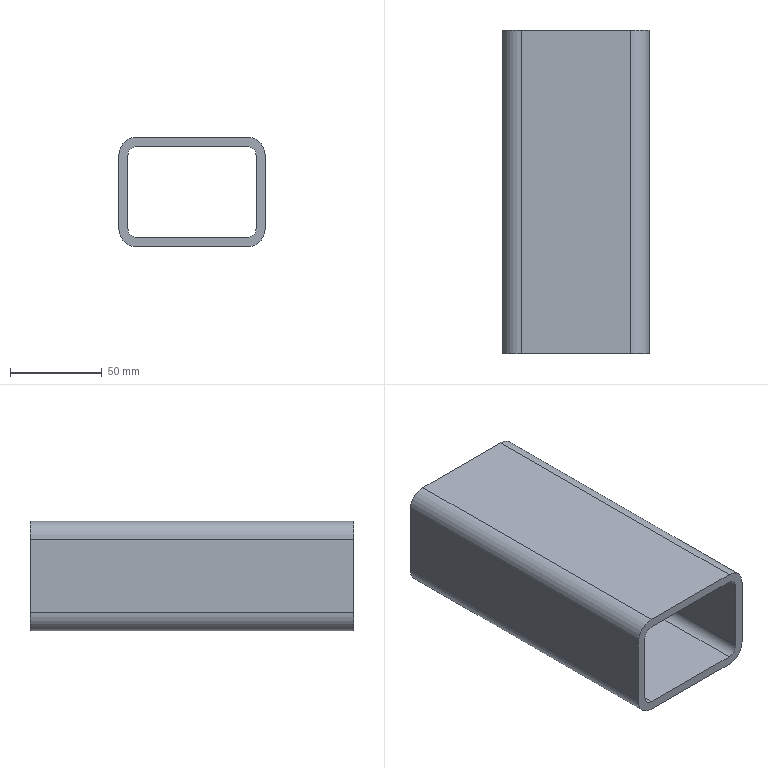Part | STEP file | front support crossmember--000.001--20240925 | 1 solid | 18 faces | box 80 x 176.5 x 60 mm | volume 218087 mm3 | plane 10 | cylinder 8 | commonest cylinder face diameters 10 x4 20 x4
STEP:
#1=CARTESIAN_POINT('',(0.,0.,0.));
#2=DIRECTION('',(0.,0.,1.));
#3=DIRECTION('',(1.,0.,0.));
#4=AXIS2_PLACEMENT_3D('',#1,#2,#3);
#5=CARTESIAN_POINT('',(10.,-176.5,40.));
#6=VERTEX_POINT('',#5);
#7=CARTESIAN_POINT('',(10.,-176.5,0.));
#8=VERTEX_POINT('',#7);
#9=CARTESIAN_POINT('',(10.,-176.5,20.));
#10=DIRECTION('',(0.,0.,-1.));
#11=VECTOR('',#10,1.);
#12=LINE('',#9,#11);
#13=CARTESIAN_POINT('',(10.,-76.5,20.));
#14=DIRECTION('',(1.,0.,0.));
#15=DIRECTION('',(0.,1.,0.));
#16=AXIS2_PLACEMENT_3D('',#13,#14,#15);
#17=PLANE('',#16);
#18=CARTESIAN_POINT('',(-100.,0.));
#19=DIRECTION('',(0.,-1.));
#20=VECTOR('',#19,1.);
#21=LINE('',#18,#20);
#22=(GEOMETRIC_REPRESENTATION_CONTEXT(2)PARAMETRIC_REPRESENTATION_CONTEXT()REPRESENTATION_CONTEXT('',''));
#23=DEFINITIONAL_REPRESENTATION('',(#21),#22);
#24=PCURVE('',#17,#23);
#25=CARTESIAN_POINT('',(-30.,-176.5,20.));
#26=DIRECTION('',(0.,-1.,0.));
#27=DIRECTION('',(1.,0.,0.));
#28=AXIS2_PLACEMENT_3D('',#25,#26,#27);
#29=PLANE('',#28);
#30=CARTESIAN_POINT('',(40.,0.));
#31=DIRECTION('',(0.,-1.));
#32=VECTOR('',#31,1.);
#33=LINE('',#30,#32);
#34=(GEOMETRIC_REPRESENTATION_CONTEXT(2)PARAMETRIC_REPRESENTATION_CONTEXT()REPRESENTATION_CONTEXT('',''));
#35=DEFINITIONAL_REPRESENTATION('',(#33),#34);
#36=PCURVE('',#29,#35);
#37=SURFACE_CURVE('',#12,(#24,#36),.PCURVE_S1.);
#38=EDGE_CURVE('',#6,#8,#37,.T.);
#39=ORIENTED_EDGE('',*,*,#38,.T.);
#40=CARTESIAN_POINT('',(10.,0.,0.));
#41=VERTEX_POINT('',#40);
#42=CARTESIAN_POINT('',(10.,-76.5,0.));
#43=DIRECTION('',(0.,1.,0.));
#44=VECTOR('',#43,1.);
#45=LINE('',#42,#44);
#46=CARTESIAN_POINT('',(0.,-20.));
#47=DIRECTION('',(1.,0.));
#48=VECTOR('',#47,1.);
#49=LINE('',#46,#48);
#50=(GEOMETRIC_REPRESENTATION_CONTEXT(2)PARAMETRIC_REPRESENTATION_CONTEXT()REPRESENTATION_CONTEXT('',''));
#51=DEFINITIONAL_REPRESENTATION('',(#49),#50);
#52=PCURVE('',#17,#51);
#53=CARTESIAN_POINT('',(0.,-76.5,0.));
#54=DIRECTION('',(0.,-1.,0.));
#55=DIRECTION('',(-0.06976,0.,-0.9976));
#56=AXIS2_PLACEMENT_3D('',#53,#54,#55);
#57=CYLINDRICAL_SURFACE('',#56,10.);
#58=CARTESIAN_POINT('',(1.641,0.));
#59=DIRECTION('',(0.,-1.));
#60=VECTOR('',#59,1.);
#61=LINE('',#58,#60);
#62=(GEOMETRIC_REPRESENTATION_CONTEXT(2)PARAMETRIC_REPRESENTATION_CONTEXT()REPRESENTATION_CONTEXT('',''));
#63=DEFINITIONAL_REPRESENTATION('',(#61),#62);
#64=PCURVE('',#57,#63);
#65=SURFACE_CURVE('',#45,(#52,#64),.PCURVE_S1.);
#66=EDGE_CURVE('',#8,#41,#65,.T.);
#67=ORIENTED_EDGE('',*,*,#66,.T.);
#68=CARTESIAN_POINT('',(10.,0.,40.));
#69=VERTEX_POINT('',#68);
#70=CARTESIAN_POINT('',(10.,0.,-87.645));
#71=DIRECTION('',(0.,0.,-1.));
#72=VECTOR('',#71,1.);
#73=LINE('',#70,#72);
#74=CARTESIAN_POINT('',(76.5,-107.645));
#75=DIRECTION('',(0.,-1.));
#76=VECTOR('',#75,1.);
#77=LINE('',#74,#76);
#78=(GEOMETRIC_REPRESENTATION_CONTEXT(2)PARAMETRIC_REPRESENTATION_CONTEXT()REPRESENTATION_CONTEXT('',''));
#79=DEFINITIONAL_REPRESENTATION('',(#77),#78);
#80=PCURVE('',#17,#79);
#81=CARTESIAN_POINT('',(131.5,0.,-87.645));
#82=DIRECTION('',(0.,1.,0.));
#83=DIRECTION('',(0.,0.,1.));
#84=AXIS2_PLACEMENT_3D('',#81,#82,#83);
#85=PLANE('',#84);
#86=CARTESIAN_POINT('',(0.,-121.5));
#87=DIRECTION('',(-1.,0.));
#88=VECTOR('',#87,1.);
#89=LINE('',#86,#88);
#90=(GEOMETRIC_REPRESENTATION_CONTEXT(2)PARAMETRIC_REPRESENTATION_CONTEXT()REPRESENTATION_CONTEXT('',''));
#91=DEFINITIONAL_REPRESENTATION('',(#89),#90);
#92=PCURVE('',#85,#91);
#93=SURFACE_CURVE('',#73,(#80,#92),.PCURVE_S1.);
#94=EDGE_CURVE('',#69,#41,#93,.T.);
#95=ORIENTED_EDGE('',*,*,#94,.F.);
#96=CARTESIAN_POINT('',(10.,-176.5,40.));
#97=DIRECTION('',(0.,-1.,0.));
#98=VECTOR('',#97,1.);
#99=LINE('',#96,#98);
#100=CARTESIAN_POINT('',(-100.,20.));
#101=DIRECTION('',(-1.,0.));
#102=VECTOR('',#101,1.);
#103=LINE('',#100,#102);
#104=(GEOMETRIC_REPRESENTATION_CONTEXT(2)PARAMETRIC_REPRESENTATION_CONTEXT()REPRESENTATION_CONTEXT('',''));
#105=DEFINITIONAL_REPRESENTATION('',(#103),#104);
#106=PCURVE('',#17,#105);
#107=CARTESIAN_POINT('',(0.,-76.5,40.));
#108=DIRECTION('',(0.,1.,0.));
#109=DIRECTION('',(0.06976,0.,0.9976));
#110=AXIS2_PLACEMENT_3D('',#107,#108,#109);
#111=CYLINDRICAL_SURFACE('',#110,10.);
#112=CARTESIAN_POINT('',(1.501,-100.));
#113=DIRECTION('',(0.,-1.));
#114=VECTOR('',#113,1.);
#115=LINE('',#112,#114);
#116=(GEOMETRIC_REPRESENTATION_CONTEXT(2)PARAMETRIC_REPRESENTATION_CONTEXT()REPRESENTATION_CONTEXT('',''));
#117=DEFINITIONAL_REPRESENTATION('',(#115),#116);
#118=PCURVE('',#111,#117);
#119=SURFACE_CURVE('',#99,(#106,#118),.PCURVE_S1.);
#120=EDGE_CURVE('',#69,#6,#119,.T.);
#121=ORIENTED_EDGE('',*,*,#120,.T.);
#122=EDGE_LOOP('',(#39,#67,#95,#121));
#123=FACE_BOUND('',#122,.T.);
#124=ADVANCED_FACE('',(#123),#17,.T.);
#125=CARTESIAN_POINT('',(-60.,-176.5,-5.));
#126=VERTEX_POINT('',#125);
#127=CARTESIAN_POINT('',(0.,-176.5,-5.));
#128=VERTEX_POINT('',#127);
#129=CARTESIAN_POINT('',(-30.,-176.5,-5.));
#130=DIRECTION('',(1.,0.,0.));
#131=VECTOR('',#130,1.);
#132=LINE('',#129,#131);
#133=CARTESIAN_POINT('',(0.,-25.));
#134=DIRECTION('',(1.,0.));
#135=VECTOR('',#134,1.);
#136=LINE('',#133,#135);
#137=(GEOMETRIC_REPRESENTATION_CONTEXT(2)PARAMETRIC_REPRESENTATION_CONTEXT()REPRESENTATION_CONTEXT('',''));
#138=DEFINITIONAL_REPRESENTATION('',(#136),#137);
#139=PCURVE('',#29,#138);
#140=CARTESIAN_POINT('',(-70.,-76.5,-5.));
#141=DIRECTION('',(0.,0.,-1.));
#142=DIRECTION('',(1.,0.,0.));
#143=AXIS2_PLACEMENT_3D('',#140,#141,#142);
#144=PLANE('',#143);
#145=CARTESIAN_POINT('',(40.,100.));
#146=DIRECTION('',(1.,0.));
#147=VECTOR('',#146,1.);
#148=LINE('',#145,#147);
#149=(GEOMETRIC_REPRESENTATION_CONTEXT(2)PARAMETRIC_REPRESENTATION_CONTEXT()REPRESENTATION_CONTEXT('',''));
#150=DEFINITIONAL_REPRESENTATION('',(#148),#149);
#151=PCURVE('',#144,#150);
#152=SURFACE_CURVE('',#132,(#139,#151),.PCURVE_S1.);
#153=EDGE_CURVE('',#126,#128,#152,.T.);
#154=ORIENTED_EDGE('',*,*,#153,.F.);
#155=CARTESIAN_POINT('',(-65.,-176.5,0.));
#156=VERTEX_POINT('',#155);
#157=CARTESIAN_POINT('',(-60.,-176.5,0.));
#158=DIRECTION('',(0.,-1.,0.));
#159=DIRECTION('',(0.06976,0.,0.9976));
#160=AXIS2_PLACEMENT_3D('',#157,#158,#159);
#161=CIRCLE('',#160,5.);
#162=CARTESIAN_POINT('',(-30.,-20.));
#163=DIRECTION('',(0.06976,0.9976));
#164=AXIS2_PLACEMENT_2D('',#162,#163);
#165=CIRCLE('',#164,5.);
#166=(GEOMETRIC_REPRESENTATION_CONTEXT(2)PARAMETRIC_REPRESENTATION_CONTEXT()REPRESENTATION_CONTEXT('',''));
#167=DEFINITIONAL_REPRESENTATION('',(#165),#166);
#168=PCURVE('',#29,#167);
#169=CARTESIAN_POINT('',(-60.,-76.5,0.));
#170=DIRECTION('',(0.,1.,0.));
#171=DIRECTION('',(0.06976,0.,0.9976));
#172=AXIS2_PLACEMENT_3D('',#169,#170,#171);
#173=CYLINDRICAL_SURFACE('',#172,5.);
#174=CARTESIAN_POINT('',(6.283,-100.));
#175=DIRECTION('',(-1.,0.));
#176=VECTOR('',#175,1.);
#177=LINE('',#174,#176);
#178=(GEOMETRIC_REPRESENTATION_CONTEXT(2)PARAMETRIC_REPRESENTATION_CONTEXT()REPRESENTATION_CONTEXT('',''));
#179=DEFINITIONAL_REPRESENTATION('',(#177),#178);
#180=PCURVE('',#173,#179);
#181=SURFACE_CURVE('',#161,(#168,#180),.PCURVE_S1.);
#182=EDGE_CURVE('',#156,#126,#181,.T.);
#183=ORIENTED_EDGE('',*,*,#182,.F.);
#184=CARTESIAN_POINT('',(-65.,-176.5,40.));
#185=VERTEX_POINT('',#184);
#186=CARTESIAN_POINT('',(-65.,-176.5,20.));
#187=DIRECTION('',(0.,0.,-1.));
#188=VECTOR('',#187,1.);
#189=LINE('',#186,#188);
#190=CARTESIAN_POINT('',(-35.,0.));
#191=DIRECTION('',(0.,-1.));
#192=VECTOR('',#191,1.);
#193=LINE('',#190,#192);
#194=(GEOMETRIC_REPRESENTATION_CONTEXT(2)PARAMETRIC_REPRESENTATION_CONTEXT()REPRESENTATION_CONTEXT('',''));
#195=DEFINITIONAL_REPRESENTATION('',(#193),#194);
#196=PCURVE('',#29,#195);
#197=CARTESIAN_POINT('',(-65.,-76.5,20.));
#198=DIRECTION('',(1.,0.,0.));
#199=DIRECTION('',(0.,1.,0.));
#200=AXIS2_PLACEMENT_3D('',#197,#198,#199);
#201=PLANE('',#200);
#202=CARTESIAN_POINT('',(-100.,0.));
#203=DIRECTION('',(0.,-1.));
#204=VECTOR('',#203,1.);
#205=LINE('',#202,#204);
#206=(GEOMETRIC_REPRESENTATION_CONTEXT(2)PARAMETRIC_REPRESENTATION_CONTEXT()REPRESENTATION_CONTEXT('',''));
#207=DEFINITIONAL_REPRESENTATION('',(#205),#206);
#208=PCURVE('',#201,#207);
#209=SURFACE_CURVE('',#189,(#196,#208),.PCURVE_S1.);
#210=EDGE_CURVE('',#185,#156,#209,.T.);
#211=ORIENTED_EDGE('',*,*,#210,.F.);
#212=CARTESIAN_POINT('',(-60.,-176.5,45.));
#213=VERTEX_POINT('',#212);
#214=CARTESIAN_POINT('',(-60.,-176.5,40.));
#215=DIRECTION('',(0.,-1.,0.));
#216=DIRECTION('',(0.06976,0.,0.9976));
#217=AXIS2_PLACEMENT_3D('',#214,#215,#216);
#218=CIRCLE('',#217,5.);
#219=CARTESIAN_POINT('',(-30.,20.));
#220=DIRECTION('',(0.06976,0.9976));
#221=AXIS2_PLACEMENT_2D('',#219,#220);
#222=CIRCLE('',#221,5.);
#223=(GEOMETRIC_REPRESENTATION_CONTEXT(2)PARAMETRIC_REPRESENTATION_CONTEXT()REPRESENTATION_CONTEXT('',''));
#224=DEFINITIONAL_REPRESENTATION('',(#222),#223);
#225=PCURVE('',#29,#224);
#226=CARTESIAN_POINT('',(-60.,-76.5,40.));
#227=DIRECTION('',(0.,-1.,0.));
#228=DIRECTION('',(-0.06976,0.,-0.9976));
#229=AXIS2_PLACEMENT_3D('',#226,#227,#228);
#230=CYLINDRICAL_SURFACE('',#229,5.);
#231=CARTESIAN_POINT('',(3.142,100.));
#232=DIRECTION('',(1.,0.));
#233=VECTOR('',#232,1.);
#234=LINE('',#231,#233);
#235=(GEOMETRIC_REPRESENTATION_CONTEXT(2)PARAMETRIC_REPRESENTATION_CONTEXT()REPRESENTATION_CONTEXT('',''));
#236=DEFINITIONAL_REPRESENTATION('',(#234),#235);
#237=PCURVE('',#230,#236);
#238=SURFACE_CURVE('',#218,(#225,#237),.PCURVE_S1.);
#239=EDGE_CURVE('',#213,#185,#238,.T.);
#240=ORIENTED_EDGE('',*,*,#239,.F.);
#241=CARTESIAN_POINT('',(0.,-176.5,45.));
#242=VERTEX_POINT('',#241);
#243=CARTESIAN_POINT('',(-30.,-176.5,45.));
#244=DIRECTION('',(1.,0.,0.));
#245=VECTOR('',#244,1.);
#246=LINE('',#243,#245);
#247=CARTESIAN_POINT('',(0.,25.));
#248=DIRECTION('',(1.,0.));
#249=VECTOR('',#248,1.);
#250=LINE('',#247,#249);
#251=(GEOMETRIC_REPRESENTATION_CONTEXT(2)PARAMETRIC_REPRESENTATION_CONTEXT()REPRESENTATION_CONTEXT('',''));
#252=DEFINITIONAL_REPRESENTATION('',(#250),#251);
#253=PCURVE('',#29,#252);
#254=CARTESIAN_POINT('',(-70.,-76.5,45.));
#255=DIRECTION('',(0.,0.,-1.));
#256=DIRECTION('',(1.,0.,0.));
#257=AXIS2_PLACEMENT_3D('',#254,#255,#256);
#258=PLANE('',#257);
#259=CARTESIAN_POINT('',(40.,100.));
#260=DIRECTION('',(1.,0.));
#261=VECTOR('',#260,1.);
#262=LINE('',#259,#261);
#263=(GEOMETRIC_REPRESENTATION_CONTEXT(2)PARAMETRIC_REPRESENTATION_CONTEXT()REPRESENTATION_CONTEXT('',''));
#264=DEFINITIONAL_REPRESENTATION('',(#262),#263);
#265=PCURVE('',#258,#264);
#266=SURFACE_CURVE('',#246,(#253,#265),.PCURVE_S1.);
#267=EDGE_CURVE('',#213,#242,#266,.T.);
#268=ORIENTED_EDGE('',*,*,#267,.T.);
#269=CARTESIAN_POINT('',(5.,-176.5,40.));
#270=VERTEX_POINT('',#269);
#271=CARTESIAN_POINT('',(0.,-176.5,40.));
#272=DIRECTION('',(0.,-1.,0.));
#273=DIRECTION('',(0.06976,0.,0.9976));
#274=AXIS2_PLACEMENT_3D('',#271,#272,#273);
#275=CIRCLE('',#274,5.);
#276=CARTESIAN_POINT('',(30.,20.));
#277=DIRECTION('',(0.06976,0.9976));
#278=AXIS2_PLACEMENT_2D('',#276,#277);
#279=CIRCLE('',#278,5.);
#280=(GEOMETRIC_REPRESENTATION_CONTEXT(2)PARAMETRIC_REPRESENTATION_CONTEXT()REPRESENTATION_CONTEXT('',''));
#281=DEFINITIONAL_REPRESENTATION('',(#279),#280);
#282=PCURVE('',#29,#281);
#283=CARTESIAN_POINT('',(0.,-76.5,40.));
#284=DIRECTION('',(0.,1.,0.));
#285=DIRECTION('',(0.06976,0.,0.9976));
#286=AXIS2_PLACEMENT_3D('',#283,#284,#285);
#287=CYLINDRICAL_SURFACE('',#286,5.);
#288=CARTESIAN_POINT('',(6.283,-100.));
#289=DIRECTION('',(-1.,0.));
#290=VECTOR('',#289,1.);
#291=LINE('',#288,#290);
#292=(GEOMETRIC_REPRESENTATION_CONTEXT(2)PARAMETRIC_REPRESENTATION_CONTEXT()REPRESENTATION_CONTEXT('',''));
#293=DEFINITIONAL_REPRESENTATION('',(#291),#292);
#294=PCURVE('',#287,#293);
#295=SURFACE_CURVE('',#275,(#282,#294),.PCURVE_S1.);
#296=EDGE_CURVE('',#270,#242,#295,.T.);
#297=ORIENTED_EDGE('',*,*,#296,.F.);
#298=CARTESIAN_POINT('',(5.,-176.5,0.));
#299=VERTEX_POINT('',#298);
#300=CARTESIAN_POINT('',(5.,-176.5,20.));
#301=DIRECTION('',(0.,0.,-1.));
#302=VECTOR('',#301,1.);
#303=LINE('',#300,#302);
#304=CARTESIAN_POINT('',(35.,0.));
#305=DIRECTION('',(0.,-1.));
#306=VECTOR('',#305,1.);
#307=LINE('',#304,#306);
#308=(GEOMETRIC_REPRESENTATION_CONTEXT(2)PARAMETRIC_REPRESENTATION_CONTEXT()REPRESENTATION_CONTEXT('',''));
#309=DEFINITIONAL_REPRESENTATION('',(#307),#308);
#310=PCURVE('',#29,#309);
#311=CARTESIAN_POINT('',(5.,-76.5,20.));
#312=DIRECTION('',(1.,0.,0.));
#313=DIRECTION('',(0.,1.,0.));
#314=AXIS2_PLACEMENT_3D('',#311,#312,#313);
#315=PLANE('',#314);
#316=CARTESIAN_POINT('',(-100.,0.));
#317=DIRECTION('',(0.,-1.));
#318=VECTOR('',#317,1.);
#319=LINE('',#316,#318);
#320=(GEOMETRIC_REPRESENTATION_CONTEXT(2)PARAMETRIC_REPRESENTATION_CONTEXT()REPRESENTATION_CONTEXT('',''));
#321=DEFINITIONAL_REPRESENTATION('',(#319),#320);
#322=PCURVE('',#315,#321);
#323=SURFACE_CURVE('',#303,(#310,#322),.PCURVE_S1.);
#324=EDGE_CURVE('',#270,#299,#323,.T.);
#325=ORIENTED_EDGE('',*,*,#324,.T.);
#326=CARTESIAN_POINT('',(0.,-176.5,0.));
#327=DIRECTION('',(0.,-1.,0.));
#328=DIRECTION('',(0.06976,0.,0.9976));
#329=AXIS2_PLACEMENT_3D('',#326,#327,#328);
#330=CIRCLE('',#329,5.);
#331=CARTESIAN_POINT('',(30.,-20.));
#332=DIRECTION('',(0.06976,0.9976));
#333=AXIS2_PLACEMENT_2D('',#331,#332);
#334=CIRCLE('',#333,5.);
#335=(GEOMETRIC_REPRESENTATION_CONTEXT(2)PARAMETRIC_REPRESENTATION_CONTEXT()REPRESENTATION_CONTEXT('',''));
#336=DEFINITIONAL_REPRESENTATION('',(#334),#335);
#337=PCURVE('',#29,#336);
#338=CARTESIAN_POINT('',(0.,-76.5,0.));
#339=DIRECTION('',(0.,-1.,0.));
#340=DIRECTION('',(-0.06976,0.,-0.9976));
#341=AXIS2_PLACEMENT_3D('',#338,#339,#340);
#342=CYLINDRICAL_SURFACE('',#341,5.);
#343=CARTESIAN_POINT('',(-3.142,100.));
#344=DIRECTION('',(1.,0.));
#345=VECTOR('',#344,1.);
#346=LINE('',#343,#345);
#347=(GEOMETRIC_REPRESENTATION_CONTEXT(2)PARAMETRIC_REPRESENTATION_CONTEXT()REPRESENTATION_CONTEXT('',''));
#348=DEFINITIONAL_REPRESENTATION('',(#346),#347);
#349=PCURVE('',#342,#348);
#350=SURFACE_CURVE('',#330,(#337,#349),.PCURVE_S1.);
#351=EDGE_CURVE('',#128,#299,#350,.T.);
#352=ORIENTED_EDGE('',*,*,#351,.F.);
#353=EDGE_LOOP('',(#154,#183,#211,#240,#268,#297,#325,#352));
#354=FACE_BOUND('',#353,.T.);
#355=CARTESIAN_POINT('',(-60.,-176.5,-10.));
#356=VERTEX_POINT('',#355);
#357=CARTESIAN_POINT('',(0.,-176.5,-10.));
#358=VERTEX_POINT('',#357);
#359=CARTESIAN_POINT('',(-30.,-176.5,-10.));
#360=DIRECTION('',(1.,0.,0.));
#361=VECTOR('',#360,1.);
#362=LINE('',#359,#361);
#363=CARTESIAN_POINT('',(0.,-30.));
#364=DIRECTION('',(1.,0.));
#365=VECTOR('',#364,1.);
#366=LINE('',#363,#365);
#367=(GEOMETRIC_REPRESENTATION_CONTEXT(2)PARAMETRIC_REPRESENTATION_CONTEXT()REPRESENTATION_CONTEXT('',''));
#368=DEFINITIONAL_REPRESENTATION('',(#366),#367);
#369=PCURVE('',#29,#368);
#370=CARTESIAN_POINT('',(-70.,-76.5,-10.));
#371=DIRECTION('',(0.,0.,-1.));
#372=DIRECTION('',(1.,0.,0.));
#373=AXIS2_PLACEMENT_3D('',#370,#371,#372);
#374=PLANE('',#373);
#375=CARTESIAN_POINT('',(40.,100.));
#376=DIRECTION('',(1.,0.));
#377=VECTOR('',#376,1.);
#378=LINE('',#375,#377);
#379=(GEOMETRIC_REPRESENTATION_CONTEXT(2)PARAMETRIC_REPRESENTATION_CONTEXT()REPRESENTATION_CONTEXT('',''));
#380=DEFINITIONAL_REPRESENTATION('',(#378),#379);
#381=PCURVE('',#374,#380);
#382=SURFACE_CURVE('',#362,(#369,#381),.PCURVE_S1.);
#383=EDGE_CURVE('',#356,#358,#382,.T.);
#384=ORIENTED_EDGE('',*,*,#383,.T.);
#385=CARTESIAN_POINT('',(0.,-176.5,0.));
#386=DIRECTION('',(0.,-1.,0.));
#387=DIRECTION('',(0.06976,0.,0.9976));
#388=AXIS2_PLACEMENT_3D('',#385,#386,#387);
#389=CIRCLE('',#388,10.);
#390=CARTESIAN_POINT('',(30.,-20.));
#391=DIRECTION('',(0.06976,0.9976));
#392=AXIS2_PLACEMENT_2D('',#390,#391);
#393=CIRCLE('',#392,10.);
#394=(GEOMETRIC_REPRESENTATION_CONTEXT(2)PARAMETRIC_REPRESENTATION_CONTEXT()REPRESENTATION_CONTEXT('',''));
#395=DEFINITIONAL_REPRESENTATION('',(#393),#394);
#396=PCURVE('',#29,#395);
#397=CARTESIAN_POINT('',(-3.142,100.));
#398=DIRECTION('',(1.,0.));
#399=VECTOR('',#398,1.);
#400=LINE('',#397,#399);
#401=(GEOMETRIC_REPRESENTATION_CONTEXT(2)PARAMETRIC_REPRESENTATION_CONTEXT()REPRESENTATION_CONTEXT('',''));
#402=DEFINITIONAL_REPRESENTATION('',(#400),#401);
#403=PCURVE('',#57,#402);
#404=SURFACE_CURVE('',#389,(#396,#403),.PCURVE_S1.);
#405=EDGE_CURVE('',#358,#8,#404,.T.);
#406=ORIENTED_EDGE('',*,*,#405,.T.);
#407=ORIENTED_EDGE('',*,*,#38,.F.);
#408=CARTESIAN_POINT('',(0.,-176.5,50.));
#409=VERTEX_POINT('',#408);
#410=CARTESIAN_POINT('',(0.,-176.5,40.));
#411=DIRECTION('',(0.,-1.,0.));
#412=DIRECTION('',(0.06976,0.,0.9976));
#413=AXIS2_PLACEMENT_3D('',#410,#411,#412);
#414=CIRCLE('',#413,10.);
#415=CARTESIAN_POINT('',(30.,20.));
#416=DIRECTION('',(0.06976,0.9976));
#417=AXIS2_PLACEMENT_2D('',#415,#416);
#418=CIRCLE('',#417,10.);
#419=(GEOMETRIC_REPRESENTATION_CONTEXT(2)PARAMETRIC_REPRESENTATION_CONTEXT()REPRESENTATION_CONTEXT('',''));
#420=DEFINITIONAL_REPRESENTATION('',(#418),#419);
#421=PCURVE('',#29,#420);
#422=CARTESIAN_POINT('',(6.283,-100.));
#423=DIRECTION('',(-1.,0.));
#424=VECTOR('',#423,1.);
#425=LINE('',#422,#424);
#426=(GEOMETRIC_REPRESENTATION_CONTEXT(2)PARAMETRIC_REPRESENTATION_CONTEXT()REPRESENTATION_CONTEXT('',''));
#427=DEFINITIONAL_REPRESENTATION('',(#425),#426);
#428=PCURVE('',#111,#427);
#429=SURFACE_CURVE('',#414,(#421,#428),.PCURVE_S1.);
#430=EDGE_CURVE('',#6,#409,#429,.T.);
#431=ORIENTED_EDGE('',*,*,#430,.T.);
#432=CARTESIAN_POINT('',(-60.,-176.5,50.));
#433=VERTEX_POINT('',#432);
#434=CARTESIAN_POINT('',(-30.,-176.5,50.));
#435=DIRECTION('',(1.,0.,0.));
#436=VECTOR('',#435,1.);
#437=LINE('',#434,#436);
#438=CARTESIAN_POINT('',(0.,30.));
#439=DIRECTION('',(1.,0.));
#440=VECTOR('',#439,1.);
#441=LINE('',#438,#440);
#442=(GEOMETRIC_REPRESENTATION_CONTEXT(2)PARAMETRIC_REPRESENTATION_CONTEXT()REPRESENTATION_CONTEXT('',''));
#443=DEFINITIONAL_REPRESENTATION('',(#441),#442);
#444=PCURVE('',#29,#443);
#445=CARTESIAN_POINT('',(-70.,-76.5,50.));
#446=DIRECTION('',(0.,0.,-1.));
#447=DIRECTION('',(1.,0.,0.));
#448=AXIS2_PLACEMENT_3D('',#445,#446,#447);
#449=PLANE('',#448);
#450=CARTESIAN_POINT('',(40.,100.));
#451=DIRECTION('',(1.,0.));
#452=VECTOR('',#451,1.);
#453=LINE('',#450,#452);
#454=(GEOMETRIC_REPRESENTATION_CONTEXT(2)PARAMETRIC_REPRESENTATION_CONTEXT()REPRESENTATION_CONTEXT('',''));
#455=DEFINITIONAL_REPRESENTATION('',(#453),#454);
#456=PCURVE('',#449,#455);
#457=SURFACE_CURVE('',#437,(#444,#456),.PCURVE_S1.);
#458=EDGE_CURVE('',#433,#409,#457,.T.);
#459=ORIENTED_EDGE('',*,*,#458,.F.);
#460=CARTESIAN_POINT('',(-70.,-176.5,40.));
#461=VERTEX_POINT('',#460);
#462=CARTESIAN_POINT('',(-60.,-176.5,40.));
#463=DIRECTION('',(0.,-1.,0.));
#464=DIRECTION('',(0.06976,0.,0.9976));
#465=AXIS2_PLACEMENT_3D('',#462,#463,#464);
#466=CIRCLE('',#465,10.);
#467=CARTESIAN_POINT('',(-30.,20.));
#468=DIRECTION('',(0.06976,0.9976));
#469=AXIS2_PLACEMENT_2D('',#467,#468);
#470=CIRCLE('',#469,10.);
#471=(GEOMETRIC_REPRESENTATION_CONTEXT(2)PARAMETRIC_REPRESENTATION_CONTEXT()REPRESENTATION_CONTEXT('',''));
#472=DEFINITIONAL_REPRESENTATION('',(#470),#471);
#473=PCURVE('',#29,#472);
#474=CARTESIAN_POINT('',(-60.,-76.5,40.));
#475=DIRECTION('',(0.,-1.,0.));
#476=DIRECTION('',(-0.06976,0.,-0.9976));
#477=AXIS2_PLACEMENT_3D('',#474,#475,#476);
#478=CYLINDRICAL_SURFACE('',#477,10.);
#479=CARTESIAN_POINT('',(3.142,100.));
#480=DIRECTION('',(1.,0.));
#481=VECTOR('',#480,1.);
#482=LINE('',#479,#481);
#483=(GEOMETRIC_REPRESENTATION_CONTEXT(2)PARAMETRIC_REPRESENTATION_CONTEXT()REPRESENTATION_CONTEXT('',''));
#484=DEFINITIONAL_REPRESENTATION('',(#482),#483);
#485=PCURVE('',#478,#484);
#486=SURFACE_CURVE('',#466,(#473,#485),.PCURVE_S1.);
#487=EDGE_CURVE('',#433,#461,#486,.T.);
#488=ORIENTED_EDGE('',*,*,#487,.T.);
#489=CARTESIAN_POINT('',(-70.,-176.5,0.));
#490=VERTEX_POINT('',#489);
#491=CARTESIAN_POINT('',(-70.,-176.5,20.));
#492=DIRECTION('',(0.,0.,-1.));
#493=VECTOR('',#492,1.);
#494=LINE('',#491,#493);
#495=CARTESIAN_POINT('',(-40.,0.));
#496=DIRECTION('',(0.,-1.));
#497=VECTOR('',#496,1.);
#498=LINE('',#495,#497);
#499=(GEOMETRIC_REPRESENTATION_CONTEXT(2)PARAMETRIC_REPRESENTATION_CONTEXT()REPRESENTATION_CONTEXT('',''));
#500=DEFINITIONAL_REPRESENTATION('',(#498),#499);
#501=PCURVE('',#29,#500);
#502=CARTESIAN_POINT('',(-70.,-76.5,20.));
#503=DIRECTION('',(1.,0.,0.));
#504=DIRECTION('',(0.,1.,0.));
#505=AXIS2_PLACEMENT_3D('',#502,#503,#504);
#506=PLANE('',#505);
#507=CARTESIAN_POINT('',(-100.,0.));
#508=DIRECTION('',(0.,-1.));
#509=VECTOR('',#508,1.);
#510=LINE('',#507,#509);
#511=(GEOMETRIC_REPRESENTATION_CONTEXT(2)PARAMETRIC_REPRESENTATION_CONTEXT()REPRESENTATION_CONTEXT('',''));
#512=DEFINITIONAL_REPRESENTATION('',(#510),#511);
#513=PCURVE('',#506,#512);
#514=SURFACE_CURVE('',#494,(#501,#513),.PCURVE_S1.);
#515=EDGE_CURVE('',#461,#490,#514,.T.);
#516=ORIENTED_EDGE('',*,*,#515,.T.);
#517=CARTESIAN_POINT('',(-60.,-176.5,0.));
#518=DIRECTION('',(0.,-1.,0.));
#519=DIRECTION('',(0.06976,0.,0.9976));
#520=AXIS2_PLACEMENT_3D('',#517,#518,#519);
#521=CIRCLE('',#520,10.);
#522=CARTESIAN_POINT('',(-30.,-20.));
#523=DIRECTION('',(0.06976,0.9976));
#524=AXIS2_PLACEMENT_2D('',#522,#523);
#525=CIRCLE('',#524,10.);
#526=(GEOMETRIC_REPRESENTATION_CONTEXT(2)PARAMETRIC_REPRESENTATION_CONTEXT()REPRESENTATION_CONTEXT('',''));
#527=DEFINITIONAL_REPRESENTATION('',(#525),#526);
#528=PCURVE('',#29,#527);
#529=CARTESIAN_POINT('',(-60.,-76.5,0.));
#530=DIRECTION('',(0.,1.,0.));
#531=DIRECTION('',(0.06976,0.,0.9976));
#532=AXIS2_PLACEMENT_3D('',#529,#530,#531);
#533=CYLINDRICAL_SURFACE('',#532,10.);
#534=CARTESIAN_POINT('',(6.283,-100.));
#535=DIRECTION('',(-1.,0.));
#536=VECTOR('',#535,1.);
#537=LINE('',#534,#536);
#538=(GEOMETRIC_REPRESENTATION_CONTEXT(2)PARAMETRIC_REPRESENTATION_CONTEXT()REPRESENTATION_CONTEXT('',''));
#539=DEFINITIONAL_REPRESENTATION('',(#537),#538);
#540=PCURVE('',#533,#539);
#541=SURFACE_CURVE('',#521,(#528,#540),.PCURVE_S1.);
#542=EDGE_CURVE('',#490,#356,#541,.T.);
#543=ORIENTED_EDGE('',*,*,#542,.T.);
#544=EDGE_LOOP('',(#384,#406,#407,#431,#459,#488,#516,#543));
#545=FACE_BOUND('',#544,.T.);
#546=ADVANCED_FACE('',(#354,#545),#29,.T.);
#547=CARTESIAN_POINT('',(-70.,0.,40.));
#548=VERTEX_POINT('',#547);
#549=CARTESIAN_POINT('',(-70.,0.,0.));
#550=VERTEX_POINT('',#549);
#551=CARTESIAN_POINT('',(-70.,0.,20.));
#552=DIRECTION('',(0.,0.,-1.));
#553=VECTOR('',#552,1.);
#554=LINE('',#551,#553);
#555=CARTESIAN_POINT('',(76.5,0.));
#556=DIRECTION('',(0.,-1.));
#557=VECTOR('',#556,1.);
#558=LINE('',#555,#557);
#559=(GEOMETRIC_REPRESENTATION_CONTEXT(2)PARAMETRIC_REPRESENTATION_CONTEXT()REPRESENTATION_CONTEXT('',''));
#560=DEFINITIONAL_REPRESENTATION('',(#558),#559);
#561=PCURVE('',#506,#560);
#562=CARTESIAN_POINT('',(107.645,-201.5));
#563=DIRECTION('',(-1.,0.));
#564=VECTOR('',#563,1.);
#565=LINE('',#562,#564);
#566=(GEOMETRIC_REPRESENTATION_CONTEXT(2)PARAMETRIC_REPRESENTATION_CONTEXT()REPRESENTATION_CONTEXT('',''));
#567=DEFINITIONAL_REPRESENTATION('',(#565),#566);
#568=PCURVE('',#85,#567);
#569=SURFACE_CURVE('',#554,(#561,#568),.PCURVE_S1.);
#570=EDGE_CURVE('',#548,#550,#569,.T.);
#571=ORIENTED_EDGE('',*,*,#570,.T.);
#572=CARTESIAN_POINT('',(-70.,-76.5,0.));
#573=DIRECTION('',(0.,-1.,0.));
#574=VECTOR('',#573,1.);
#575=LINE('',#572,#574);
#576=CARTESIAN_POINT('',(0.,-20.));
#577=DIRECTION('',(-1.,0.));
#578=VECTOR('',#577,1.);
#579=LINE('',#576,#578);
#580=(GEOMETRIC_REPRESENTATION_CONTEXT(2)PARAMETRIC_REPRESENTATION_CONTEXT()REPRESENTATION_CONTEXT('',''));
#581=DEFINITIONAL_REPRESENTATION('',(#579),#580);
#582=PCURVE('',#506,#581);
#583=CARTESIAN_POINT('',(4.643,0.));
#584=DIRECTION('',(0.,-1.));
#585=VECTOR('',#584,1.);
#586=LINE('',#583,#585);
#587=(GEOMETRIC_REPRESENTATION_CONTEXT(2)PARAMETRIC_REPRESENTATION_CONTEXT()REPRESENTATION_CONTEXT('',''));
#588=DEFINITIONAL_REPRESENTATION('',(#586),#587);
#589=PCURVE('',#533,#588);
#590=SURFACE_CURVE('',#575,(#582,#589),.PCURVE_S1.);
#591=EDGE_CURVE('',#550,#490,#590,.T.);
#592=ORIENTED_EDGE('',*,*,#591,.T.);
#593=ORIENTED_EDGE('',*,*,#515,.F.);
#594=CARTESIAN_POINT('',(-70.,-76.5,40.));
#595=DIRECTION('',(0.,1.,0.));
#596=VECTOR('',#595,1.);
#597=LINE('',#594,#596);
#598=CARTESIAN_POINT('',(0.,20.));
#599=DIRECTION('',(1.,0.));
#600=VECTOR('',#599,1.);
#601=LINE('',#598,#600);
#602=(GEOMETRIC_REPRESENTATION_CONTEXT(2)PARAMETRIC_REPRESENTATION_CONTEXT()REPRESENTATION_CONTEXT('',''));
#603=DEFINITIONAL_REPRESENTATION('',(#601),#602);
#604=PCURVE('',#506,#603);
#605=CARTESIAN_POINT('',(4.782,0.));
#606=DIRECTION('',(0.,-1.));
#607=VECTOR('',#606,1.);
#608=LINE('',#605,#607);
#609=(GEOMETRIC_REPRESENTATION_CONTEXT(2)PARAMETRIC_REPRESENTATION_CONTEXT()REPRESENTATION_CONTEXT('',''));
#610=DEFINITIONAL_REPRESENTATION('',(#608),#609);
#611=PCURVE('',#478,#610);
#612=SURFACE_CURVE('',#597,(#604,#611),.PCURVE_S1.);
#613=EDGE_CURVE('',#461,#548,#612,.T.);
#614=ORIENTED_EDGE('',*,*,#613,.T.);
#615=EDGE_LOOP('',(#571,#592,#593,#614));
#616=FACE_BOUND('',#615,.T.);
#617=ADVANCED_FACE('',(#616),#506,.F.);
#618=CARTESIAN_POINT('',(5.,0.,40.));
#619=VERTEX_POINT('',#618);
#620=CARTESIAN_POINT('',(5.,0.,0.));
#621=VERTEX_POINT('',#620);
#622=CARTESIAN_POINT('',(5.,0.,-87.645));
#623=DIRECTION('',(0.,0.,-1.));
#624=VECTOR('',#623,1.);
#625=LINE('',#622,#624);
#626=CARTESIAN_POINT('',(0.,-126.5));
#627=DIRECTION('',(-1.,0.));
#628=VECTOR('',#627,1.);
#629=LINE('',#626,#628);
#630=(GEOMETRIC_REPRESENTATION_CONTEXT(2)PARAMETRIC_REPRESENTATION_CONTEXT()REPRESENTATION_CONTEXT('',''));
#631=DEFINITIONAL_REPRESENTATION('',(#629),#630);
#632=PCURVE('',#85,#631);
#633=CARTESIAN_POINT('',(76.5,-107.645));
#634=DIRECTION('',(0.,-1.));
#635=VECTOR('',#634,1.);
#636=LINE('',#633,#635);
#637=(GEOMETRIC_REPRESENTATION_CONTEXT(2)PARAMETRIC_REPRESENTATION_CONTEXT()REPRESENTATION_CONTEXT('',''));
#638=DEFINITIONAL_REPRESENTATION('',(#636),#637);
#639=PCURVE('',#315,#638);
#640=SURFACE_CURVE('',#625,(#632,#639),.PCURVE_S1.);
#641=EDGE_CURVE('',#619,#621,#640,.T.);
#642=ORIENTED_EDGE('',*,*,#641,.F.);
#643=CARTESIAN_POINT('',(0.,0.,45.));
#644=VERTEX_POINT('',#643);
#645=CARTESIAN_POINT('',(0.,0.,40.));
#646=DIRECTION('',(0.,1.,0.));
#647=DIRECTION('',(-0.06976,0.,-0.9976));
#648=AXIS2_PLACEMENT_3D('',#645,#646,#647);
#649=CIRCLE('',#648,5.);
#650=CARTESIAN_POINT('',(127.645,-131.5));
#651=DIRECTION('',(-0.9976,-0.06976));
#652=AXIS2_PLACEMENT_2D('',#650,#651);
#653=CIRCLE('',#652,5.);
#654=(GEOMETRIC_REPRESENTATION_CONTEXT(2)PARAMETRIC_REPRESENTATION_CONTEXT()REPRESENTATION_CONTEXT('',''));
#655=DEFINITIONAL_REPRESENTATION('',(#653),#654);
#656=PCURVE('',#85,#655);
#657=CARTESIAN_POINT('',(-3.142,76.5));
#658=DIRECTION('',(1.,0.));
#659=VECTOR('',#658,1.);
#660=LINE('',#657,#659);
#661=(GEOMETRIC_REPRESENTATION_CONTEXT(2)PARAMETRIC_REPRESENTATION_CONTEXT()REPRESENTATION_CONTEXT('',''));
#662=DEFINITIONAL_REPRESENTATION('',(#660),#661);
#663=PCURVE('',#287,#662);
#664=SURFACE_CURVE('',#649,(#656,#663),.PCURVE_S1.);
#665=EDGE_CURVE('',#644,#619,#664,.T.);
#666=ORIENTED_EDGE('',*,*,#665,.F.);
#667=CARTESIAN_POINT('',(-60.,0.,45.));
#668=VERTEX_POINT('',#667);
#669=CARTESIAN_POINT('',(131.5,0.,45.));
#670=DIRECTION('',(-1.,0.,0.));
#671=VECTOR('',#670,1.);
#672=LINE('',#669,#671);
#673=CARTESIAN_POINT('',(132.645,0.));
#674=DIRECTION('',(0.,-1.));
#675=VECTOR('',#674,1.);
#676=LINE('',#673,#675);
#677=(GEOMETRIC_REPRESENTATION_CONTEXT(2)PARAMETRIC_REPRESENTATION_CONTEXT()REPRESENTATION_CONTEXT('',''));
#678=DEFINITIONAL_REPRESENTATION('',(#676),#677);
#679=PCURVE('',#85,#678);
#680=CARTESIAN_POINT('',(201.5,-76.5));
#681=DIRECTION('',(-1.,0.));
#682=VECTOR('',#681,1.);
#683=LINE('',#680,#682);
#684=(GEOMETRIC_REPRESENTATION_CONTEXT(2)PARAMETRIC_REPRESENTATION_CONTEXT()REPRESENTATION_CONTEXT('',''));
#685=DEFINITIONAL_REPRESENTATION('',(#683),#684);
#686=PCURVE('',#258,#685);
#687=SURFACE_CURVE('',#672,(#679,#686),.PCURVE_S1.);
#688=EDGE_CURVE('',#644,#668,#687,.T.);
#689=ORIENTED_EDGE('',*,*,#688,.T.);
#690=CARTESIAN_POINT('',(-65.,0.,40.));
#691=VERTEX_POINT('',#690);
#692=CARTESIAN_POINT('',(-60.,0.,40.));
#693=DIRECTION('',(0.,1.,0.));
#694=DIRECTION('',(-0.06976,0.,-0.9976));
#695=AXIS2_PLACEMENT_3D('',#692,#693,#694);
#696=CIRCLE('',#695,5.);
#697=CARTESIAN_POINT('',(127.645,-191.5));
#698=DIRECTION('',(-0.9976,-0.06976));
#699=AXIS2_PLACEMENT_2D('',#697,#698);
#700=CIRCLE('',#699,5.);
#701=(GEOMETRIC_REPRESENTATION_CONTEXT(2)PARAMETRIC_REPRESENTATION_CONTEXT()REPRESENTATION_CONTEXT('',''));
#702=DEFINITIONAL_REPRESENTATION('',(#700),#701);
#703=PCURVE('',#85,#702);
#704=CARTESIAN_POINT('',(6.283,-76.5));
#705=DIRECTION('',(-1.,0.));
#706=VECTOR('',#705,1.);
#707=LINE('',#704,#706);
#708=(GEOMETRIC_REPRESENTATION_CONTEXT(2)PARAMETRIC_REPRESENTATION_CONTEXT()REPRESENTATION_CONTEXT('',''));
#709=DEFINITIONAL_REPRESENTATION('',(#707),#708);
#710=PCURVE('',#230,#709);
#711=SURFACE_CURVE('',#696,(#703,#710),.PCURVE_S1.);
#712=EDGE_CURVE('',#691,#668,#711,.T.);
#713=ORIENTED_EDGE('',*,*,#712,.F.);
#714=CARTESIAN_POINT('',(-65.,0.,0.));
#715=VERTEX_POINT('',#714);
#716=CARTESIAN_POINT('',(-65.,0.,20.));
#717=DIRECTION('',(0.,0.,-1.));
#718=VECTOR('',#717,1.);
#719=LINE('',#716,#718);
#720=CARTESIAN_POINT('',(107.645,-196.5));
#721=DIRECTION('',(-1.,0.));
#722=VECTOR('',#721,1.);
#723=LINE('',#720,#722);
#724=(GEOMETRIC_REPRESENTATION_CONTEXT(2)PARAMETRIC_REPRESENTATION_CONTEXT()REPRESENTATION_CONTEXT('',''));
#725=DEFINITIONAL_REPRESENTATION('',(#723),#724);
#726=PCURVE('',#85,#725);
#727=CARTESIAN_POINT('',(76.5,0.));
#728=DIRECTION('',(0.,-1.));
#729=VECTOR('',#728,1.);
#730=LINE('',#727,#729);
#731=(GEOMETRIC_REPRESENTATION_CONTEXT(2)PARAMETRIC_REPRESENTATION_CONTEXT()REPRESENTATION_CONTEXT('',''));
#732=DEFINITIONAL_REPRESENTATION('',(#730),#731);
#733=PCURVE('',#201,#732);
#734=SURFACE_CURVE('',#719,(#726,#733),.PCURVE_S1.);
#735=EDGE_CURVE('',#691,#715,#734,.T.);
#736=ORIENTED_EDGE('',*,*,#735,.T.);
#737=CARTESIAN_POINT('',(-60.,0.,-5.));
#738=VERTEX_POINT('',#737);
#739=CARTESIAN_POINT('',(-60.,0.,0.));
#740=DIRECTION('',(0.,1.,0.));
#741=DIRECTION('',(-0.06976,0.,-0.9976));
#742=AXIS2_PLACEMENT_3D('',#739,#740,#741);
#743=CIRCLE('',#742,5.);
#744=CARTESIAN_POINT('',(87.645,-191.5));
#745=DIRECTION('',(-0.9976,-0.06976));
#746=AXIS2_PLACEMENT_2D('',#744,#745);
#747=CIRCLE('',#746,5.);
#748=(GEOMETRIC_REPRESENTATION_CONTEXT(2)PARAMETRIC_REPRESENTATION_CONTEXT()REPRESENTATION_CONTEXT('',''));
#749=DEFINITIONAL_REPRESENTATION('',(#747),#748);
#750=PCURVE('',#85,#749);
#751=CARTESIAN_POINT('',(-3.142,76.5));
#752=DIRECTION('',(1.,0.));
#753=VECTOR('',#752,1.);
#754=LINE('',#751,#753);
#755=(GEOMETRIC_REPRESENTATION_CONTEXT(2)PARAMETRIC_REPRESENTATION_CONTEXT()REPRESENTATION_CONTEXT('',''));
#756=DEFINITIONAL_REPRESENTATION('',(#754),#755);
#757=PCURVE('',#173,#756);
#758=SURFACE_CURVE('',#743,(#750,#757),.PCURVE_S1.);
#759=EDGE_CURVE('',#738,#715,#758,.T.);
#760=ORIENTED_EDGE('',*,*,#759,.F.);
#761=CARTESIAN_POINT('',(0.,0.,-5.));
#762=VERTEX_POINT('',#761);
#763=CARTESIAN_POINT('',(131.5,0.,-5.));
#764=DIRECTION('',(-1.,0.,0.));
#765=VECTOR('',#764,1.);
#766=LINE('',#763,#765);
#767=CARTESIAN_POINT('',(82.645,0.));
#768=DIRECTION('',(0.,-1.));
#769=VECTOR('',#768,1.);
#770=LINE('',#767,#769);
#771=(GEOMETRIC_REPRESENTATION_CONTEXT(2)PARAMETRIC_REPRESENTATION_CONTEXT()REPRESENTATION_CONTEXT('',''));
#772=DEFINITIONAL_REPRESENTATION('',(#770),#771);
#773=PCURVE('',#85,#772);
#774=CARTESIAN_POINT('',(201.5,-76.5));
#775=DIRECTION('',(-1.,0.));
#776=VECTOR('',#775,1.);
#777=LINE('',#774,#776);
#778=(GEOMETRIC_REPRESENTATION_CONTEXT(2)PARAMETRIC_REPRESENTATION_CONTEXT()REPRESENTATION_CONTEXT('',''));
#779=DEFINITIONAL_REPRESENTATION('',(#777),#778);
#780=PCURVE('',#144,#779);
#781=SURFACE_CURVE('',#766,(#773,#780),.PCURVE_S1.);
#782=EDGE_CURVE('',#762,#738,#781,.T.);
#783=ORIENTED_EDGE('',*,*,#782,.F.);
#784=CARTESIAN_POINT('',(0.,0.,0.));
#785=DIRECTION('',(0.,1.,0.));
#786=DIRECTION('',(-0.06976,0.,-0.9976));
#787=AXIS2_PLACEMENT_3D('',#784,#785,#786);
#788=CIRCLE('',#787,5.);
#789=CARTESIAN_POINT('',(87.645,-131.5));
#790=DIRECTION('',(-0.9976,-0.06976));
#791=AXIS2_PLACEMENT_2D('',#789,#790);
#792=CIRCLE('',#791,5.);
#793=(GEOMETRIC_REPRESENTATION_CONTEXT(2)PARAMETRIC_REPRESENTATION_CONTEXT()REPRESENTATION_CONTEXT('',''));
#794=DEFINITIONAL_REPRESENTATION('',(#792),#793);
#795=PCURVE('',#85,#794);
#796=CARTESIAN_POINT('',(6.283,-76.5));
#797=DIRECTION('',(-1.,0.));
#798=VECTOR('',#797,1.);
#799=LINE('',#796,#798);
#800=(GEOMETRIC_REPRESENTATION_CONTEXT(2)PARAMETRIC_REPRESENTATION_CONTEXT()REPRESENTATION_CONTEXT('',''));
#801=DEFINITIONAL_REPRESENTATION('',(#799),#800);
#802=PCURVE('',#342,#801);
#803=SURFACE_CURVE('',#788,(#795,#802),.PCURVE_S1.);
#804=EDGE_CURVE('',#621,#762,#803,.T.);
#805=ORIENTED_EDGE('',*,*,#804,.F.);
#806=EDGE_LOOP('',(#642,#666,#689,#713,#736,#760,#783,#805));
#807=FACE_BOUND('',#806,.T.);
#808=ORIENTED_EDGE('',*,*,#94,.T.);
#809=CARTESIAN_POINT('',(0.,0.,-10.));
#810=VERTEX_POINT('',#809);
#811=CARTESIAN_POINT('',(0.,0.,0.));
#812=DIRECTION('',(0.,1.,0.));
#813=DIRECTION('',(-0.06976,0.,-0.9976));
#814=AXIS2_PLACEMENT_3D('',#811,#812,#813);
#815=CIRCLE('',#814,10.);
#816=CARTESIAN_POINT('',(87.645,-131.5));
#817=DIRECTION('',(-0.9976,-0.06976));
#818=AXIS2_PLACEMENT_2D('',#816,#817);
#819=CIRCLE('',#818,10.);
#820=(GEOMETRIC_REPRESENTATION_CONTEXT(2)PARAMETRIC_REPRESENTATION_CONTEXT()REPRESENTATION_CONTEXT('',''));
#821=DEFINITIONAL_REPRESENTATION('',(#819),#820);
#822=PCURVE('',#85,#821);
#823=CARTESIAN_POINT('',(6.283,-76.5));
#824=DIRECTION('',(-1.,0.));
#825=VECTOR('',#824,1.);
#826=LINE('',#823,#825);
#827=(GEOMETRIC_REPRESENTATION_CONTEXT(2)PARAMETRIC_REPRESENTATION_CONTEXT()REPRESENTATION_CONTEXT('',''));
#828=DEFINITIONAL_REPRESENTATION('',(#826),#827);
#829=PCURVE('',#57,#828);
#830=SURFACE_CURVE('',#815,(#822,#829),.PCURVE_S1.);
#831=EDGE_CURVE('',#41,#810,#830,.T.);
#832=ORIENTED_EDGE('',*,*,#831,.T.);
#833=CARTESIAN_POINT('',(-60.,0.,-10.));
#834=VERTEX_POINT('',#833);
#835=CARTESIAN_POINT('',(131.5,0.,-10.));
#836=DIRECTION('',(-1.,0.,0.));
#837=VECTOR('',#836,1.);
#838=LINE('',#835,#837);
#839=CARTESIAN_POINT('',(77.645,0.));
#840=DIRECTION('',(0.,-1.));
#841=VECTOR('',#840,1.);
#842=LINE('',#839,#841);
#843=(GEOMETRIC_REPRESENTATION_CONTEXT(2)PARAMETRIC_REPRESENTATION_CONTEXT()REPRESENTATION_CONTEXT('',''));
#844=DEFINITIONAL_REPRESENTATION('',(#842),#843);
#845=PCURVE('',#85,#844);
#846=CARTESIAN_POINT('',(201.5,-76.5));
#847=DIRECTION('',(-1.,0.));
#848=VECTOR('',#847,1.);
#849=LINE('',#846,#848);
#850=(GEOMETRIC_REPRESENTATION_CONTEXT(2)PARAMETRIC_REPRESENTATION_CONTEXT()REPRESENTATION_CONTEXT('',''));
#851=DEFINITIONAL_REPRESENTATION('',(#849),#850);
#852=PCURVE('',#374,#851);
#853=SURFACE_CURVE('',#838,(#845,#852),.PCURVE_S1.);
#854=EDGE_CURVE('',#810,#834,#853,.T.);
#855=ORIENTED_EDGE('',*,*,#854,.T.);
#856=CARTESIAN_POINT('',(-60.,0.,0.));
#857=DIRECTION('',(0.,1.,0.));
#858=DIRECTION('',(-0.06976,0.,-0.9976));
#859=AXIS2_PLACEMENT_3D('',#856,#857,#858);
#860=CIRCLE('',#859,10.);
#861=CARTESIAN_POINT('',(87.645,-191.5));
#862=DIRECTION('',(-0.9976,-0.06976));
#863=AXIS2_PLACEMENT_2D('',#861,#862);
#864=CIRCLE('',#863,10.);
#865=(GEOMETRIC_REPRESENTATION_CONTEXT(2)PARAMETRIC_REPRESENTATION_CONTEXT()REPRESENTATION_CONTEXT('',''));
#866=DEFINITIONAL_REPRESENTATION('',(#864),#865);
#867=PCURVE('',#85,#866);
#868=CARTESIAN_POINT('',(-3.142,76.5));
#869=DIRECTION('',(1.,0.));
#870=VECTOR('',#869,1.);
#871=LINE('',#868,#870);
#872=(GEOMETRIC_REPRESENTATION_CONTEXT(2)PARAMETRIC_REPRESENTATION_CONTEXT()REPRESENTATION_CONTEXT('',''));
#873=DEFINITIONAL_REPRESENTATION('',(#871),#872);
#874=PCURVE('',#533,#873);
#875=SURFACE_CURVE('',#860,(#867,#874),.PCURVE_S1.);
#876=EDGE_CURVE('',#834,#550,#875,.T.);
#877=ORIENTED_EDGE('',*,*,#876,.T.);
#878=ORIENTED_EDGE('',*,*,#570,.F.);
#879=CARTESIAN_POINT('',(-60.,0.,50.));
#880=VERTEX_POINT('',#879);
#881=CARTESIAN_POINT('',(-60.,0.,40.));
#882=DIRECTION('',(0.,1.,0.));
#883=DIRECTION('',(-0.06976,0.,-0.9976));
#884=AXIS2_PLACEMENT_3D('',#881,#882,#883);
#885=CIRCLE('',#884,10.);
#886=CARTESIAN_POINT('',(127.645,-191.5));
#887=DIRECTION('',(-0.9976,-0.06976));
#888=AXIS2_PLACEMENT_2D('',#886,#887);
#889=CIRCLE('',#888,10.);
#890=(GEOMETRIC_REPRESENTATION_CONTEXT(2)PARAMETRIC_REPRESENTATION_CONTEXT()REPRESENTATION_CONTEXT('',''));
#891=DEFINITIONAL_REPRESENTATION('',(#889),#890);
#892=PCURVE('',#85,#891);
#893=CARTESIAN_POINT('',(6.283,-76.5));
#894=DIRECTION('',(-1.,0.));
#895=VECTOR('',#894,1.);
#896=LINE('',#893,#895);
#897=(GEOMETRIC_REPRESENTATION_CONTEXT(2)PARAMETRIC_REPRESENTATION_CONTEXT()REPRESENTATION_CONTEXT('',''));
#898=DEFINITIONAL_REPRESENTATION('',(#896),#897);
#899=PCURVE('',#478,#898);
#900=SURFACE_CURVE('',#885,(#892,#899),.PCURVE_S1.);
#901=EDGE_CURVE('',#548,#880,#900,.T.);
#902=ORIENTED_EDGE('',*,*,#901,.T.);
#903=CARTESIAN_POINT('',(0.,0.,50.));
#904=VERTEX_POINT('',#903);
#905=CARTESIAN_POINT('',(131.5,0.,50.));
#906=DIRECTION('',(-1.,0.,0.));
#907=VECTOR('',#906,1.);
#908=LINE('',#905,#907);
#909=CARTESIAN_POINT('',(137.645,0.));
#910=DIRECTION('',(0.,-1.));
#911=VECTOR('',#910,1.);
#912=LINE('',#909,#911);
#913=(GEOMETRIC_REPRESENTATION_CONTEXT(2)PARAMETRIC_REPRESENTATION_CONTEXT()REPRESENTATION_CONTEXT('',''));
#914=DEFINITIONAL_REPRESENTATION('',(#912),#913);
#915=PCURVE('',#85,#914);
#916=CARTESIAN_POINT('',(201.5,-76.5));
#917=DIRECTION('',(-1.,0.));
#918=VECTOR('',#917,1.);
#919=LINE('',#916,#918);
#920=(GEOMETRIC_REPRESENTATION_CONTEXT(2)PARAMETRIC_REPRESENTATION_CONTEXT()REPRESENTATION_CONTEXT('',''));
#921=DEFINITIONAL_REPRESENTATION('',(#919),#920);
#922=PCURVE('',#449,#921);
#923=SURFACE_CURVE('',#908,(#915,#922),.PCURVE_S1.);
#924=EDGE_CURVE('',#904,#880,#923,.T.);
#925=ORIENTED_EDGE('',*,*,#924,.F.);
#926=CARTESIAN_POINT('',(0.,0.,40.));
#927=DIRECTION('',(0.,1.,0.));
#928=DIRECTION('',(-0.06976,0.,-0.9976));
#929=AXIS2_PLACEMENT_3D('',#926,#927,#928);
#930=CIRCLE('',#929,10.);
#931=CARTESIAN_POINT('',(127.645,-131.5));
#932=DIRECTION('',(-0.9976,-0.06976));
#933=AXIS2_PLACEMENT_2D('',#931,#932);
#934=CIRCLE('',#933,10.);
#935=(GEOMETRIC_REPRESENTATION_CONTEXT(2)PARAMETRIC_REPRESENTATION_CONTEXT()REPRESENTATION_CONTEXT('',''));
#936=DEFINITIONAL_REPRESENTATION('',(#934),#935);
#937=PCURVE('',#85,#936);
#938=CARTESIAN_POINT('',(-3.142,76.5));
#939=DIRECTION('',(1.,0.));
#940=VECTOR('',#939,1.);
#941=LINE('',#938,#940);
#942=(GEOMETRIC_REPRESENTATION_CONTEXT(2)PARAMETRIC_REPRESENTATION_CONTEXT()REPRESENTATION_CONTEXT('',''));
#943=DEFINITIONAL_REPRESENTATION('',(#941),#942);
#944=PCURVE('',#111,#943);
#945=SURFACE_CURVE('',#930,(#937,#944),.PCURVE_S1.);
#946=EDGE_CURVE('',#904,#69,#945,.T.);
#947=ORIENTED_EDGE('',*,*,#946,.T.);
#948=EDGE_LOOP('',(#808,#832,#855,#877,#878,#902,#925,#947));
#949=FACE_BOUND('',#948,.T.);
#950=ADVANCED_FACE('',(#807,#949),#85,.T.);
#951=ORIENTED_EDGE('',*,*,#854,.F.);
#952=CARTESIAN_POINT('',(0.,-76.5,-10.));
#953=DIRECTION('',(0.,-1.,0.));
#954=VECTOR('',#953,1.);
#955=LINE('',#952,#954);
#956=CARTESIAN_POINT('',(70.,0.));
#957=DIRECTION('',(0.,1.));
#958=VECTOR('',#957,1.);
#959=LINE('',#956,#958);
#960=(GEOMETRIC_REPRESENTATION_CONTEXT(2)PARAMETRIC_REPRESENTATION_CONTEXT()REPRESENTATION_CONTEXT('',''));
#961=DEFINITIONAL_REPRESENTATION('',(#959),#960);
#962=PCURVE('',#374,#961);
#963=CARTESIAN_POINT('',(0.06981,0.));
#964=DIRECTION('',(0.,1.));
#965=VECTOR('',#964,1.);
#966=LINE('',#963,#965);
#967=(GEOMETRIC_REPRESENTATION_CONTEXT(2)PARAMETRIC_REPRESENTATION_CONTEXT()REPRESENTATION_CONTEXT('',''));
#968=DEFINITIONAL_REPRESENTATION('',(#966),#967);
#969=PCURVE('',#57,#968);
#970=SURFACE_CURVE('',#955,(#962,#969),.PCURVE_S1.);
#971=EDGE_CURVE('',#810,#358,#970,.T.);
#972=ORIENTED_EDGE('',*,*,#971,.T.);
#973=ORIENTED_EDGE('',*,*,#383,.F.);
#974=CARTESIAN_POINT('',(-60.,-76.5,-10.));
#975=DIRECTION('',(0.,1.,0.));
#976=VECTOR('',#975,1.);
#977=LINE('',#974,#976);
#978=CARTESIAN_POINT('',(10.,0.));
#979=DIRECTION('',(0.,-1.));
#980=VECTOR('',#979,1.);
#981=LINE('',#978,#980);
#982=(GEOMETRIC_REPRESENTATION_CONTEXT(2)PARAMETRIC_REPRESENTATION_CONTEXT()REPRESENTATION_CONTEXT('',''));
#983=DEFINITIONAL_REPRESENTATION('',(#981),#982);
#984=PCURVE('',#374,#983);
#985=CARTESIAN_POINT('',(3.072,0.));
#986=DIRECTION('',(0.,1.));
#987=VECTOR('',#986,1.);
#988=LINE('',#985,#987);
#989=(GEOMETRIC_REPRESENTATION_CONTEXT(2)PARAMETRIC_REPRESENTATION_CONTEXT()REPRESENTATION_CONTEXT('',''));
#990=DEFINITIONAL_REPRESENTATION('',(#988),#989);
#991=PCURVE('',#533,#990);
#992=SURFACE_CURVE('',#977,(#984,#991),.PCURVE_S1.);
#993=EDGE_CURVE('',#356,#834,#992,.T.);
#994=ORIENTED_EDGE('',*,*,#993,.T.);
#995=EDGE_LOOP('',(#951,#972,#973,#994));
#996=FACE_BOUND('',#995,.T.);
#997=ADVANCED_FACE('',(#996),#374,.T.);
#998=ORIENTED_EDGE('',*,*,#458,.T.);
#999=CARTESIAN_POINT('',(0.,-76.5,50.));
#1000=DIRECTION('',(0.,1.,0.));
#1001=VECTOR('',#1000,1.);
#1002=LINE('',#999,#1001);
#1003=CARTESIAN_POINT('',(70.,0.));
#1004=DIRECTION('',(0.,-1.));
#1005=VECTOR('',#1004,1.);
#1006=LINE('',#1003,#1005);
#1007=(GEOMETRIC_REPRESENTATION_CONTEXT(2)PARAMETRIC_REPRESENTATION_CONTEXT()REPRESENTATION_CONTEXT('',''));
#1008=DEFINITIONAL_REPRESENTATION('',(#1006),#1007);
#1009=PCURVE('',#449,#1008);
#1010=CARTESIAN_POINT('',(-0.06981,0.));
#1011=DIRECTION('',(0.,1.));
#1012=VECTOR('',#1011,1.);
#1013=LINE('',#1010,#1012);
#1014=(GEOMETRIC_REPRESENTATION_CONTEXT(2)PARAMETRIC_REPRESENTATION_CONTEXT()REPRESENTATION_CONTEXT('',''));
#1015=DEFINITIONAL_REPRESENTATION('',(#1013),#1014);
#1016=PCURVE('',#111,#1015);
#1017=SURFACE_CURVE('',#1002,(#1009,#1016),.PCURVE_S1.);
#1018=EDGE_CURVE('',#409,#904,#1017,.T.);
#1019=ORIENTED_EDGE('',*,*,#1018,.T.);
#1020=ORIENTED_EDGE('',*,*,#924,.T.);
#1021=CARTESIAN_POINT('',(-60.,-176.5,50.));
#1022=DIRECTION('',(0.,-1.,0.));
#1023=VECTOR('',#1022,1.);
#1024=LINE('',#1021,#1023);
#1025=CARTESIAN_POINT('',(10.,100.));
#1026=DIRECTION('',(0.,1.));
#1027=VECTOR('',#1026,1.);
#1028=LINE('',#1025,#1027);
#1029=(GEOMETRIC_REPRESENTATION_CONTEXT(2)PARAMETRIC_REPRESENTATION_CONTEXT()REPRESENTATION_CONTEXT('',''));
#1030=DEFINITIONAL_REPRESENTATION('',(#1028),#1029);
#1031=PCURVE('',#449,#1030);
#1032=CARTESIAN_POINT('',(3.211,100.));
#1033=DIRECTION('',(0.,1.));
#1034=VECTOR('',#1033,1.);
#1035=LINE('',#1032,#1034);
#1036=(GEOMETRIC_REPRESENTATION_CONTEXT(2)PARAMETRIC_REPRESENTATION_CONTEXT()REPRESENTATION_CONTEXT('',''));
#1037=DEFINITIONAL_REPRESENTATION('',(#1035),#1036);
#1038=PCURVE('',#478,#1037);
#1039=SURFACE_CURVE('',#1024,(#1031,#1038),.PCURVE_S1.);
#1040=EDGE_CURVE('',#880,#433,#1039,.T.);
#1041=ORIENTED_EDGE('',*,*,#1040,.T.);
#1042=EDGE_LOOP('',(#998,#1019,#1020,#1041));
#1043=FACE_BOUND('',#1042,.T.);
#1044=ADVANCED_FACE('',(#1043),#449,.F.);
#1045=ORIENTED_EDGE('',*,*,#831,.F.);
#1046=ORIENTED_EDGE('',*,*,#66,.F.);
#1047=ORIENTED_EDGE('',*,*,#405,.F.);
#1048=ORIENTED_EDGE('',*,*,#971,.F.);
#1049=EDGE_LOOP('',(#1045,#1046,#1047,#1048));
#1050=FACE_BOUND('',#1049,.T.);
#1051=ADVANCED_FACE('',(#1050),#57,.T.);
#1052=ORIENTED_EDGE('',*,*,#946,.F.);
#1053=ORIENTED_EDGE('',*,*,#1018,.F.);
#1054=ORIENTED_EDGE('',*,*,#430,.F.);
#1055=ORIENTED_EDGE('',*,*,#120,.F.);
#1056=EDGE_LOOP('',(#1052,#1053,#1054,#1055));
#1057=FACE_BOUND('',#1056,.T.);
#1058=ADVANCED_FACE('',(#1057),#111,.T.);
#1059=ORIENTED_EDGE('',*,*,#876,.F.);
#1060=ORIENTED_EDGE('',*,*,#993,.F.);
#1061=ORIENTED_EDGE('',*,*,#542,.F.);
#1062=ORIENTED_EDGE('',*,*,#591,.F.);
#1063=EDGE_LOOP('',(#1059,#1060,#1061,#1062));
#1064=FACE_BOUND('',#1063,.T.);
#1065=ADVANCED_FACE('',(#1064),#533,.T.);
#1066=ORIENTED_EDGE('',*,*,#901,.F.);
#1067=ORIENTED_EDGE('',*,*,#613,.F.);
#1068=ORIENTED_EDGE('',*,*,#487,.F.);
#1069=ORIENTED_EDGE('',*,*,#1040,.F.);
#1070=EDGE_LOOP('',(#1066,#1067,#1068,#1069));
#1071=FACE_BOUND('',#1070,.T.);
#1072=ADVANCED_FACE('',(#1071),#478,.T.);
#1073=ORIENTED_EDGE('',*,*,#324,.F.);
#1074=CARTESIAN_POINT('',(5.,-76.5,40.));
#1075=DIRECTION('',(0.,-1.,0.));
#1076=VECTOR('',#1075,1.);
#1077=LINE('',#1074,#1076);
#1078=CARTESIAN_POINT('',(0.,20.));
#1079=DIRECTION('',(-1.,0.));
#1080=VECTOR('',#1079,1.);
#1081=LINE('',#1078,#1080);
#1082=(GEOMETRIC_REPRESENTATION_CONTEXT(2)PARAMETRIC_REPRESENTATION_CONTEXT()REPRESENTATION_CONTEXT('',''));
#1083=DEFINITIONAL_REPRESENTATION('',(#1081),#1082);
#1084=PCURVE('',#315,#1083);
#1085=CARTESIAN_POINT('',(1.501,0.));
#1086=DIRECTION('',(0.,-1.));
#1087=VECTOR('',#1086,1.);
#1088=LINE('',#1085,#1087);
#1089=(GEOMETRIC_REPRESENTATION_CONTEXT(2)PARAMETRIC_REPRESENTATION_CONTEXT()REPRESENTATION_CONTEXT('',''));
#1090=DEFINITIONAL_REPRESENTATION('',(#1088),#1089);
#1091=PCURVE('',#287,#1090);
#1092=SURFACE_CURVE('',#1077,(#1084,#1091),.PCURVE_S1.);
#1093=EDGE_CURVE('',#619,#270,#1092,.T.);
#1094=ORIENTED_EDGE('',*,*,#1093,.F.);
#1095=ORIENTED_EDGE('',*,*,#641,.T.);
#1096=CARTESIAN_POINT('',(5.,-76.5,0.));
#1097=DIRECTION('',(0.,1.,0.));
#1098=VECTOR('',#1097,1.);
#1099=LINE('',#1096,#1098);
#1100=CARTESIAN_POINT('',(0.,-20.));
#1101=DIRECTION('',(1.,0.));
#1102=VECTOR('',#1101,1.);
#1103=LINE('',#1100,#1102);
#1104=(GEOMETRIC_REPRESENTATION_CONTEXT(2)PARAMETRIC_REPRESENTATION_CONTEXT()REPRESENTATION_CONTEXT('',''));
#1105=DEFINITIONAL_REPRESENTATION('',(#1103),#1104);
#1106=PCURVE('',#315,#1105);
#1107=CARTESIAN_POINT('',(1.641,0.));
#1108=DIRECTION('',(0.,-1.));
#1109=VECTOR('',#1108,1.);
#1110=LINE('',#1107,#1109);
#1111=(GEOMETRIC_REPRESENTATION_CONTEXT(2)PARAMETRIC_REPRESENTATION_CONTEXT()REPRESENTATION_CONTEXT('',''));
#1112=DEFINITIONAL_REPRESENTATION('',(#1110),#1111);
#1113=PCURVE('',#342,#1112);
#1114=SURFACE_CURVE('',#1099,(#1106,#1113),.PCURVE_S1.);
#1115=EDGE_CURVE('',#299,#621,#1114,.T.);
#1116=ORIENTED_EDGE('',*,*,#1115,.F.);
#1117=EDGE_LOOP('',(#1073,#1094,#1095,#1116));
#1118=FACE_BOUND('',#1117,.T.);
#1119=ADVANCED_FACE('',(#1118),#315,.F.);
#1120=ORIENTED_EDGE('',*,*,#735,.F.);
#1121=CARTESIAN_POINT('',(-65.,-76.5,40.));
#1122=DIRECTION('',(0.,1.,0.));
#1123=VECTOR('',#1122,1.);
#1124=LINE('',#1121,#1123);
#1125=CARTESIAN_POINT('',(0.,20.));
#1126=DIRECTION('',(1.,0.));
#1127=VECTOR('',#1126,1.);
#1128=LINE('',#1125,#1127);
#1129=(GEOMETRIC_REPRESENTATION_CONTEXT(2)PARAMETRIC_REPRESENTATION_CONTEXT()REPRESENTATION_CONTEXT('',''));
#1130=DEFINITIONAL_REPRESENTATION('',(#1128),#1129);
#1131=PCURVE('',#201,#1130);
#1132=CARTESIAN_POINT('',(4.782,0.));
#1133=DIRECTION('',(0.,-1.));
#1134=VECTOR('',#1133,1.);
#1135=LINE('',#1132,#1134);
#1136=(GEOMETRIC_REPRESENTATION_CONTEXT(2)PARAMETRIC_REPRESENTATION_CONTEXT()REPRESENTATION_CONTEXT('',''));
#1137=DEFINITIONAL_REPRESENTATION('',(#1135),#1136);
#1138=PCURVE('',#230,#1137);
#1139=SURFACE_CURVE('',#1124,(#1131,#1138),.PCURVE_S1.);
#1140=EDGE_CURVE('',#185,#691,#1139,.T.);
#1141=ORIENTED_EDGE('',*,*,#1140,.F.);
#1142=ORIENTED_EDGE('',*,*,#210,.T.);
#1143=CARTESIAN_POINT('',(-65.,-76.5,0.));
#1144=DIRECTION('',(0.,-1.,0.));
#1145=VECTOR('',#1144,1.);
#1146=LINE('',#1143,#1145);
#1147=CARTESIAN_POINT('',(0.,-20.));
#1148=DIRECTION('',(-1.,0.));
#1149=VECTOR('',#1148,1.);
#1150=LINE('',#1147,#1149);
#1151=(GEOMETRIC_REPRESENTATION_CONTEXT(2)PARAMETRIC_REPRESENTATION_CONTEXT()REPRESENTATION_CONTEXT('',''));
#1152=DEFINITIONAL_REPRESENTATION('',(#1150),#1151);
#1153=PCURVE('',#201,#1152);
#1154=CARTESIAN_POINT('',(4.643,0.));
#1155=DIRECTION('',(0.,-1.));
#1156=VECTOR('',#1155,1.);
#1157=LINE('',#1154,#1156);
#1158=(GEOMETRIC_REPRESENTATION_CONTEXT(2)PARAMETRIC_REPRESENTATION_CONTEXT()REPRESENTATION_CONTEXT('',''));
#1159=DEFINITIONAL_REPRESENTATION('',(#1157),#1158);
#1160=PCURVE('',#173,#1159);
#1161=SURFACE_CURVE('',#1146,(#1153,#1160),.PCURVE_S1.);
#1162=EDGE_CURVE('',#715,#156,#1161,.T.);
#1163=ORIENTED_EDGE('',*,*,#1162,.F.);
#1164=EDGE_LOOP('',(#1120,#1141,#1142,#1163));
#1165=FACE_BOUND('',#1164,.T.);
#1166=ADVANCED_FACE('',(#1165),#201,.T.);
#1167=ORIENTED_EDGE('',*,*,#782,.T.);
#1168=CARTESIAN_POINT('',(-60.,-76.5,-5.));
#1169=DIRECTION('',(0.,1.,0.));
#1170=VECTOR('',#1169,1.);
#1171=LINE('',#1168,#1170);
#1172=CARTESIAN_POINT('',(10.,0.));
#1173=DIRECTION('',(0.,-1.));
#1174=VECTOR('',#1173,1.);
#1175=LINE('',#1172,#1174);
#1176=(GEOMETRIC_REPRESENTATION_CONTEXT(2)PARAMETRIC_REPRESENTATION_CONTEXT()REPRESENTATION_CONTEXT('',''));
#1177=DEFINITIONAL_REPRESENTATION('',(#1175),#1176);
#1178=PCURVE('',#144,#1177);
#1179=CARTESIAN_POINT('',(3.072,0.));
#1180=DIRECTION('',(0.,1.));
#1181=VECTOR('',#1180,1.);
#1182=LINE('',#1179,#1181);
#1183=(GEOMETRIC_REPRESENTATION_CONTEXT(2)PARAMETRIC_REPRESENTATION_CONTEXT()REPRESENTATION_CONTEXT('',''));
#1184=DEFINITIONAL_REPRESENTATION('',(#1182),#1183);
#1185=PCURVE('',#173,#1184);
#1186=SURFACE_CURVE('',#1171,(#1178,#1185),.PCURVE_S1.);
#1187=EDGE_CURVE('',#126,#738,#1186,.T.);
#1188=ORIENTED_EDGE('',*,*,#1187,.F.);
#1189=ORIENTED_EDGE('',*,*,#153,.T.);
#1190=CARTESIAN_POINT('',(0.,-76.5,-5.));
#1191=DIRECTION('',(0.,-1.,0.));
#1192=VECTOR('',#1191,1.);
#1193=LINE('',#1190,#1192);
#1194=CARTESIAN_POINT('',(70.,0.));
#1195=DIRECTION('',(0.,1.));
#1196=VECTOR('',#1195,1.);
#1197=LINE('',#1194,#1196);
#1198=(GEOMETRIC_REPRESENTATION_CONTEXT(2)PARAMETRIC_REPRESENTATION_CONTEXT()REPRESENTATION_CONTEXT('',''));
#1199=DEFINITIONAL_REPRESENTATION('',(#1197),#1198);
#1200=PCURVE('',#144,#1199);
#1201=CARTESIAN_POINT('',(0.06981,0.));
#1202=DIRECTION('',(0.,1.));
#1203=VECTOR('',#1202,1.);
#1204=LINE('',#1201,#1203);
#1205=(GEOMETRIC_REPRESENTATION_CONTEXT(2)PARAMETRIC_REPRESENTATION_CONTEXT()REPRESENTATION_CONTEXT('',''));
#1206=DEFINITIONAL_REPRESENTATION('',(#1204),#1205);
#1207=PCURVE('',#342,#1206);
#1208=SURFACE_CURVE('',#1193,(#1200,#1207),.PCURVE_S1.);
#1209=EDGE_CURVE('',#762,#128,#1208,.T.);
#1210=ORIENTED_EDGE('',*,*,#1209,.F.);
#1211=EDGE_LOOP('',(#1167,#1188,#1189,#1210));
#1212=FACE_BOUND('',#1211,.T.);
#1213=ADVANCED_FACE('',(#1212),#144,.F.);
#1214=ORIENTED_EDGE('',*,*,#267,.F.);
#1215=CARTESIAN_POINT('',(-60.,-76.5,45.));
#1216=DIRECTION('',(0.,-1.,0.));
#1217=VECTOR('',#1216,1.);
#1218=LINE('',#1215,#1217);
#1219=CARTESIAN_POINT('',(10.,0.));
#1220=DIRECTION('',(0.,1.));
#1221=VECTOR('',#1220,1.);
#1222=LINE('',#1219,#1221);
#1223=(GEOMETRIC_REPRESENTATION_CONTEXT(2)PARAMETRIC_REPRESENTATION_CONTEXT()REPRESENTATION_CONTEXT('',''));
#1224=DEFINITIONAL_REPRESENTATION('',(#1222),#1223);
#1225=PCURVE('',#258,#1224);
#1226=CARTESIAN_POINT('',(3.211,0.));
#1227=DIRECTION('',(0.,1.));
#1228=VECTOR('',#1227,1.);
#1229=LINE('',#1226,#1228);
#1230=(GEOMETRIC_REPRESENTATION_CONTEXT(2)PARAMETRIC_REPRESENTATION_CONTEXT()REPRESENTATION_CONTEXT('',''));
#1231=DEFINITIONAL_REPRESENTATION('',(#1229),#1230);
#1232=PCURVE('',#230,#1231);
#1233=SURFACE_CURVE('',#1218,(#1225,#1232),.PCURVE_S1.);
#1234=EDGE_CURVE('',#668,#213,#1233,.T.);
#1235=ORIENTED_EDGE('',*,*,#1234,.F.);
#1236=ORIENTED_EDGE('',*,*,#688,.F.);
#1237=CARTESIAN_POINT('',(0.,-76.5,45.));
#1238=DIRECTION('',(0.,1.,0.));
#1239=VECTOR('',#1238,1.);
#1240=LINE('',#1237,#1239);
#1241=CARTESIAN_POINT('',(70.,0.));
#1242=DIRECTION('',(0.,-1.));
#1243=VECTOR('',#1242,1.);
#1244=LINE('',#1241,#1243);
#1245=(GEOMETRIC_REPRESENTATION_CONTEXT(2)PARAMETRIC_REPRESENTATION_CONTEXT()REPRESENTATION_CONTEXT('',''));
#1246=DEFINITIONAL_REPRESENTATION('',(#1244),#1245);
#1247=PCURVE('',#258,#1246);
#1248=CARTESIAN_POINT('',(-0.06981,0.));
#1249=DIRECTION('',(0.,1.));
#1250=VECTOR('',#1249,1.);
#1251=LINE('',#1248,#1250);
#1252=(GEOMETRIC_REPRESENTATION_CONTEXT(2)PARAMETRIC_REPRESENTATION_CONTEXT()REPRESENTATION_CONTEXT('',''));
#1253=DEFINITIONAL_REPRESENTATION('',(#1251),#1252);
#1254=PCURVE('',#287,#1253);
#1255=SURFACE_CURVE('',#1240,(#1247,#1254),.PCURVE_S1.);
#1256=EDGE_CURVE('',#242,#644,#1255,.T.);
#1257=ORIENTED_EDGE('',*,*,#1256,.F.);
#1258=EDGE_LOOP('',(#1214,#1235,#1236,#1257));
#1259=FACE_BOUND('',#1258,.T.);
#1260=ADVANCED_FACE('',(#1259),#258,.T.);
#1261=ORIENTED_EDGE('',*,*,#1115,.F.);
#1262=ORIENTED_EDGE('',*,*,#351,.F.);
#1263=ORIENTED_EDGE('',*,*,#1209,.F.);
#1264=ORIENTED_EDGE('',*,*,#804,.F.);
#1265=EDGE_LOOP('',(#1261,#1262,#1263,#1264));
#1266=FACE_BOUND('',#1265,.F.);
#1267=ADVANCED_FACE('',(#1266),#342,.F.);
#1268=ORIENTED_EDGE('',*,*,#1256,.F.);
#1269=ORIENTED_EDGE('',*,*,#296,.F.);
#1270=ORIENTED_EDGE('',*,*,#1093,.F.);
#1271=ORIENTED_EDGE('',*,*,#665,.F.);
#1272=EDGE_LOOP('',(#1268,#1269,#1270,#1271));
#1273=FACE_BOUND('',#1272,.F.);
#1274=ADVANCED_FACE('',(#1273),#287,.F.);
#1275=ORIENTED_EDGE('',*,*,#1187,.F.);
#1276=ORIENTED_EDGE('',*,*,#182,.F.);
#1277=ORIENTED_EDGE('',*,*,#1162,.F.);
#1278=ORIENTED_EDGE('',*,*,#759,.F.);
#1279=EDGE_LOOP('',(#1275,#1276,#1277,#1278));
#1280=FACE_BOUND('',#1279,.F.);
#1281=ADVANCED_FACE('',(#1280),#173,.F.);
#1282=ORIENTED_EDGE('',*,*,#1140,.F.);
#1283=ORIENTED_EDGE('',*,*,#239,.F.);
#1284=ORIENTED_EDGE('',*,*,#1234,.F.);
#1285=ORIENTED_EDGE('',*,*,#712,.F.);
#1286=EDGE_LOOP('',(#1282,#1283,#1284,#1285));
#1287=FACE_BOUND('',#1286,.F.);
#1288=ADVANCED_FACE('',(#1287),#230,.F.);
#1289=CLOSED_SHELL('',(#124,#546,#617,#950,#997,#1044,#1051,#1058,#1065,#1072,#1119,#1166,#1213,#1260,#1267,#1274,#1281,#1288));
#1290=MANIFOLD_SOLID_BREP('',#1289);
#1291=(LENGTH_UNIT()NAMED_UNIT(*)SI_UNIT(.MILLI.,.METRE.));
#1292=UNCERTAINTY_MEASURE_WITH_UNIT(LENGTH_MEASURE(0.0000001),#1291,'','');
#1293=(NAMED_UNIT(*)PLANE_ANGLE_UNIT()SI_UNIT($,.RADIAN.));
#1294=(NAMED_UNIT(*)SI_UNIT($,.STERADIAN.)SOLID_ANGLE_UNIT());
#1295=(GEOMETRIC_REPRESENTATION_CONTEXT(3)GLOBAL_UNCERTAINTY_ASSIGNED_CONTEXT((#1292))GLOBAL_UNIT_ASSIGNED_CONTEXT((#1291,#1293,#1294))REPRESENTATION_CONTEXT('',''));
#1296=ADVANCED_BREP_SHAPE_REPRESENTATION('',(#4,#1290),#1295);